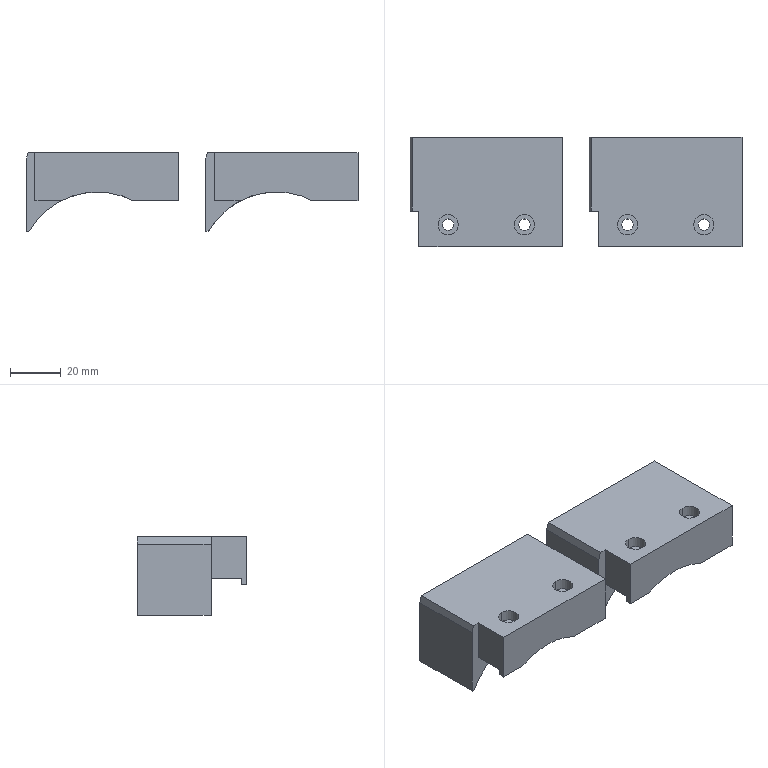Part | 2 solids | 58 faces | box 130.5 x 43 x 31 mm | volume 90954 mm3 | plane 38 | cylinder 20 | commonest cylinder face diameters 4.5 x8 8 x8 62 x4